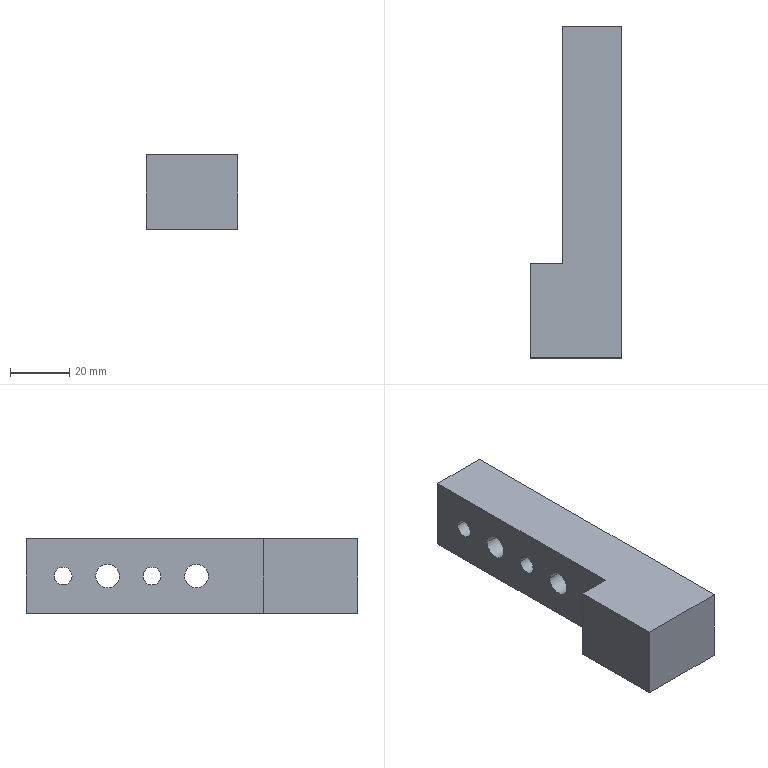Part | STEP file | Positioning_id1702_x_t | 1 solid | 16 faces | box 30.998 x 111.963 x 25 mm | volume 61638 mm3 | cylinder 8 | plane 8 | commonest cylinder face diameters 6 x4 8 x4